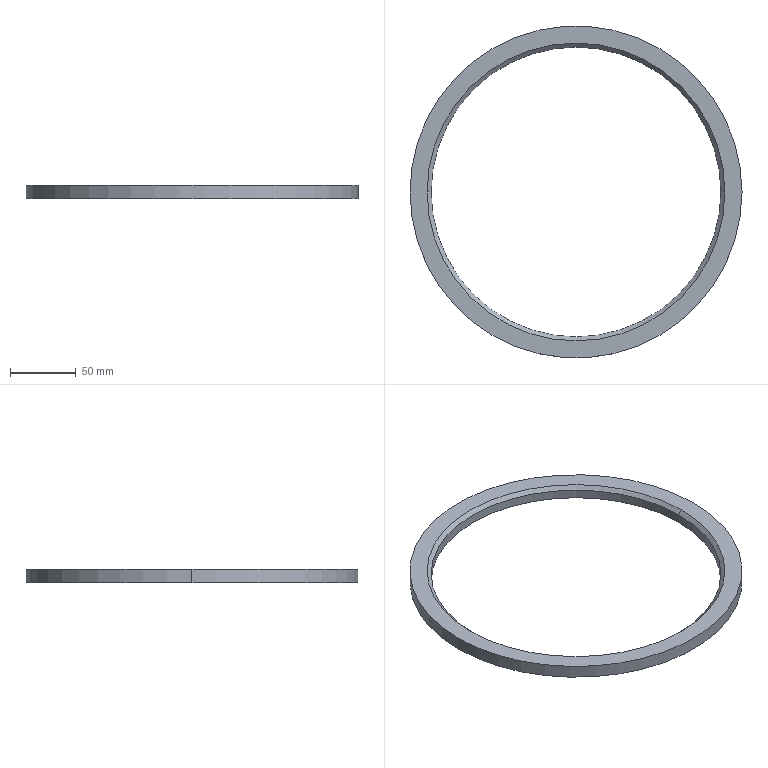Part | SolidWorks | features Chamfer 1, Extrusion 1 | 1 solid | 8 faces | box 252 x 252 x 10 mm | volume 115488 mm3 | cylinder 4 | cone 2 | plane 2 | commonest cylinder face diameters 220 x2 252 x2
STEP:
#1=CARTESIAN_POINT('',(-110.,0.,7.));
#2=VERTEX_POINT('',#1);
#3=CARTESIAN_POINT('',(110.,0.,7.));
#4=VERTEX_POINT('',#3);
#5=CARTESIAN_POINT('',(0.,0.,7.));
#6=DIRECTION('',(0.,0.,1.));
#7=DIRECTION('',(1.,0.,0.));
#8=AXIS2_PLACEMENT_3D('',#5,#6,#7);
#9=CIRCLE('',#8,110.);
#10=EDGE_CURVE('',#2,#4,#9,.T.);
#11=ORIENTED_EDGE('',*,*,#10,.F.);
#12=CARTESIAN_POINT('',(-113.,0.,10.));
#13=VERTEX_POINT('',#12);
#14=CARTESIAN_POINT('',(-110.,0.,7.));
#15=DIRECTION('',(-0.7071,0.,0.7071));
#16=VECTOR('',#15,1000.);
#17=LINE('',#14,#16);
#18=EDGE_CURVE('',#2,#13,#17,.T.);
#19=ORIENTED_EDGE('',*,*,#18,.T.);
#20=CARTESIAN_POINT('',(113.,0.,10.));
#21=VERTEX_POINT('',#20);
#22=CARTESIAN_POINT('',(0.,0.,10.));
#23=DIRECTION('',(0.,0.,-1.));
#24=DIRECTION('',(1.,0.,0.));
#25=AXIS2_PLACEMENT_3D('',#22,#23,#24);
#26=CIRCLE('',#25,113.);
#27=EDGE_CURVE('',#21,#13,#26,.T.);
#28=ORIENTED_EDGE('',*,*,#27,.F.);
#29=CARTESIAN_POINT('',(110.,0.,7.));
#30=DIRECTION('',(0.7071,0.,0.7071));
#31=VECTOR('',#30,1000.);
#32=LINE('',#29,#31);
#33=EDGE_CURVE('',#4,#21,#32,.T.);
#34=ORIENTED_EDGE('',*,*,#33,.F.);
#35=EDGE_LOOP('',(#11,#19,#28,#34));
#36=FACE_OUTER_BOUND('',#35,.T.);
#37=CARTESIAN_POINT('',(0.,0.,7.));
#38=DIRECTION('',(0.,0.,1.));
#39=DIRECTION('',(1.,0.,0.));
#40=AXIS2_PLACEMENT_3D('',#37,#38,#39);
#41=CONICAL_SURFACE('',#40,110.,0.7854);
#42=ADVANCED_FACE('',(#36),#41,.F.);
#43=ORIENTED_EDGE('',*,*,#10,.T.);
#44=CARTESIAN_POINT('',(110.,0.,0.));
#45=VERTEX_POINT('',#44);
#46=CARTESIAN_POINT('',(110.,0.,10.));
#47=DIRECTION('',(0.,0.,-1.));
#48=VECTOR('',#47,1000.);
#49=LINE('',#46,#48);
#50=EDGE_CURVE('',#4,#45,#49,.T.);
#51=ORIENTED_EDGE('',*,*,#50,.T.);
#52=CARTESIAN_POINT('',(-110.,0.,0.));
#53=VERTEX_POINT('',#52);
#54=CARTESIAN_POINT('',(0.,0.,0.));
#55=DIRECTION('',(0.,0.,1.));
#56=DIRECTION('',(1.,0.,0.));
#57=AXIS2_PLACEMENT_3D('',#54,#55,#56);
#58=CIRCLE('',#57,110.);
#59=EDGE_CURVE('',#53,#45,#58,.T.);
#60=ORIENTED_EDGE('',*,*,#59,.F.);
#61=CARTESIAN_POINT('',(-110.,0.,10.));
#62=DIRECTION('',(0.,0.,-1.));
#63=VECTOR('',#62,1000.);
#64=LINE('',#61,#63);
#65=EDGE_CURVE('',#2,#53,#64,.T.);
#66=ORIENTED_EDGE('',*,*,#65,.F.);
#67=EDGE_LOOP('',(#43,#51,#60,#66));
#68=FACE_OUTER_BOUND('',#67,.T.);
#69=CARTESIAN_POINT('',(0.,0.,10.));
#70=DIRECTION('',(0.,0.,-1.));
#71=DIRECTION('',(-1.,0.,0.));
#72=AXIS2_PLACEMENT_3D('',#69,#70,#71);
#73=CYLINDRICAL_SURFACE('',#72,110.);
#74=ADVANCED_FACE('',(#68),#73,.F.);
#75=CARTESIAN_POINT('',(126.,0.,10.));
#76=VERTEX_POINT('',#75);
#77=CARTESIAN_POINT('',(-126.,0.,10.));
#78=VERTEX_POINT('',#77);
#79=CARTESIAN_POINT('',(0.,0.,10.));
#80=DIRECTION('',(0.,0.,1.));
#81=DIRECTION('',(1.,0.,0.));
#82=AXIS2_PLACEMENT_3D('',#79,#80,#81);
#83=CIRCLE('',#82,126.);
#84=EDGE_CURVE('',#76,#78,#83,.T.);
#85=ORIENTED_EDGE('',*,*,#84,.F.);
#86=CARTESIAN_POINT('',(126.,0.,0.));
#87=VERTEX_POINT('',#86);
#88=CARTESIAN_POINT('',(126.,0.,10.));
#89=DIRECTION('',(0.,0.,-1.));
#90=VECTOR('',#89,1000.);
#91=LINE('',#88,#90);
#92=EDGE_CURVE('',#76,#87,#91,.T.);
#93=ORIENTED_EDGE('',*,*,#92,.T.);
#94=CARTESIAN_POINT('',(-126.,0.,0.));
#95=VERTEX_POINT('',#94);
#96=CARTESIAN_POINT('',(0.,0.,0.));
#97=DIRECTION('',(0.,0.,1.));
#98=DIRECTION('',(1.,0.,0.));
#99=AXIS2_PLACEMENT_3D('',#96,#97,#98);
#100=CIRCLE('',#99,126.);
#101=EDGE_CURVE('',#87,#95,#100,.T.);
#102=ORIENTED_EDGE('',*,*,#101,.T.);
#103=CARTESIAN_POINT('',(-126.,0.,10.));
#104=DIRECTION('',(0.,0.,-1.));
#105=VECTOR('',#104,1000.);
#106=LINE('',#103,#105);
#107=EDGE_CURVE('',#78,#95,#106,.T.);
#108=ORIENTED_EDGE('',*,*,#107,.F.);
#109=EDGE_LOOP('',(#85,#93,#102,#108));
#110=FACE_OUTER_BOUND('',#109,.T.);
#111=CARTESIAN_POINT('',(0.,0.,10.));
#112=DIRECTION('',(0.,0.,-1.));
#113=DIRECTION('',(-1.,0.,0.));
#114=AXIS2_PLACEMENT_3D('',#111,#112,#113);
#115=CYLINDRICAL_SURFACE('',#114,126.);
#116=ADVANCED_FACE('',(#110),#115,.T.);
#117=ORIENTED_EDGE('',*,*,#27,.T.);
#118=CARTESIAN_POINT('',(0.,0.,10.));
#119=DIRECTION('',(0.,0.,-1.));
#120=DIRECTION('',(1.,0.,0.));
#121=AXIS2_PLACEMENT_3D('',#118,#119,#120);
#122=CIRCLE('',#121,113.);
#123=EDGE_CURVE('',#13,#21,#122,.T.);
#124=ORIENTED_EDGE('',*,*,#123,.T.);
#125=EDGE_LOOP('',(#117,#124));
#126=FACE_BOUND('',#125,.T.);
#127=CARTESIAN_POINT('',(0.,0.,10.));
#128=DIRECTION('',(0.,0.,1.));
#129=DIRECTION('',(1.,0.,0.));
#130=AXIS2_PLACEMENT_3D('',#127,#128,#129);
#131=CIRCLE('',#130,126.);
#132=EDGE_CURVE('',#78,#76,#131,.T.);
#133=ORIENTED_EDGE('',*,*,#132,.T.);
#134=ORIENTED_EDGE('',*,*,#84,.T.);
#135=EDGE_LOOP('',(#133,#134));
#136=FACE_OUTER_BOUND('',#135,.T.);
#137=CARTESIAN_POINT('',(0.,0.,10.));
#138=DIRECTION('',(0.,0.,1.));
#139=DIRECTION('',(1.,0.,0.));
#140=AXIS2_PLACEMENT_3D('',#137,#138,#139);
#141=PLANE('',#140);
#142=ADVANCED_FACE('',(#126,#136),#141,.T.);
#143=CARTESIAN_POINT('',(0.,0.,0.));
#144=DIRECTION('',(0.,0.,1.));
#145=DIRECTION('',(1.,0.,0.));
#146=AXIS2_PLACEMENT_3D('',#143,#144,#145);
#147=CIRCLE('',#146,126.);
#148=EDGE_CURVE('',#95,#87,#147,.T.);
#149=ORIENTED_EDGE('',*,*,#148,.F.);
#150=ORIENTED_EDGE('',*,*,#101,.F.);
#151=EDGE_LOOP('',(#149,#150));
#152=FACE_OUTER_BOUND('',#151,.T.);
#153=ORIENTED_EDGE('',*,*,#59,.T.);
#154=CARTESIAN_POINT('',(0.,0.,0.));
#155=DIRECTION('',(0.,0.,1.));
#156=DIRECTION('',(1.,0.,0.));
#157=AXIS2_PLACEMENT_3D('',#154,#155,#156);
#158=CIRCLE('',#157,110.);
#159=EDGE_CURVE('',#45,#53,#158,.T.);
#160=ORIENTED_EDGE('',*,*,#159,.T.);
#161=EDGE_LOOP('',(#153,#160));
#162=FACE_BOUND('',#161,.T.);
#163=CARTESIAN_POINT('',(0.,0.,0.));
#164=DIRECTION('',(0.,0.,1.));
#165=DIRECTION('',(1.,0.,0.));
#166=AXIS2_PLACEMENT_3D('',#163,#164,#165);
#167=PLANE('',#166);
#168=ADVANCED_FACE('',(#152,#162),#167,.F.);
#169=ORIENTED_EDGE('',*,*,#92,.F.);
#170=ORIENTED_EDGE('',*,*,#132,.F.);
#171=ORIENTED_EDGE('',*,*,#107,.T.);
#172=ORIENTED_EDGE('',*,*,#148,.T.);
#173=EDGE_LOOP('',(#169,#170,#171,#172));
#174=FACE_OUTER_BOUND('',#173,.T.);
#175=CARTESIAN_POINT('',(0.,0.,10.));
#176=DIRECTION('',(0.,0.,-1.));
#177=DIRECTION('',(-1.,0.,0.));
#178=AXIS2_PLACEMENT_3D('',#175,#176,#177);
#179=CYLINDRICAL_SURFACE('',#178,126.);
#180=ADVANCED_FACE('',(#174),#179,.T.);
#181=ORIENTED_EDGE('',*,*,#50,.F.);
#182=CARTESIAN_POINT('',(0.,0.,7.));
#183=DIRECTION('',(0.,0.,1.));
#184=DIRECTION('',(1.,0.,0.));
#185=AXIS2_PLACEMENT_3D('',#182,#183,#184);
#186=CIRCLE('',#185,110.);
#187=EDGE_CURVE('',#4,#2,#186,.T.);
#188=ORIENTED_EDGE('',*,*,#187,.T.);
#189=ORIENTED_EDGE('',*,*,#65,.T.);
#190=ORIENTED_EDGE('',*,*,#159,.F.);
#191=EDGE_LOOP('',(#181,#188,#189,#190));
#192=FACE_OUTER_BOUND('',#191,.T.);
#193=CARTESIAN_POINT('',(0.,0.,10.));
#194=DIRECTION('',(0.,0.,-1.));
#195=DIRECTION('',(-1.,0.,0.));
#196=AXIS2_PLACEMENT_3D('',#193,#194,#195);
#197=CYLINDRICAL_SURFACE('',#196,110.);
#198=ADVANCED_FACE('',(#192),#197,.F.);
#199=ORIENTED_EDGE('',*,*,#18,.F.);
#200=ORIENTED_EDGE('',*,*,#187,.F.);
#201=ORIENTED_EDGE('',*,*,#33,.T.);
#202=ORIENTED_EDGE('',*,*,#123,.F.);
#203=EDGE_LOOP('',(#199,#200,#201,#202));
#204=FACE_OUTER_BOUND('',#203,.T.);
#205=CARTESIAN_POINT('',(0.,0.,7.));
#206=DIRECTION('',(0.,0.,1.));
#207=DIRECTION('',(1.,0.,0.));
#208=AXIS2_PLACEMENT_3D('',#205,#206,#207);
#209=CONICAL_SURFACE('',#208,110.,0.7854);
#210=ADVANCED_FACE('',(#204),#209,.F.);
#211=CLOSED_SHELL('',(#42,#74,#116,#142,#168,#180,#198,#210));
#212=MANIFOLD_SOLID_BREP('',#211);
#213=CARTESIAN_POINT('',(0.,0.,0.));
#214=DIRECTION('',(0.,0.,1.));
#215=DIRECTION('',(1.,0.,0.));
#216=AXIS2_PLACEMENT_3D('',#213,#214,#215);
#217=(LENGTH_UNIT()NAMED_UNIT(*)SI_UNIT(.MILLI.,.METRE.));
#218=UNCERTAINTY_MEASURE_WITH_UNIT(LENGTH_MEASURE(0.00001),#217,'','');
#219=(NAMED_UNIT(*)PLANE_ANGLE_UNIT()SI_UNIT($,.RADIAN.));
#220=(NAMED_UNIT(*)SI_UNIT($,.STERADIAN.)SOLID_ANGLE_UNIT());
#221=(GEOMETRIC_REPRESENTATION_CONTEXT(3)GLOBAL_UNCERTAINTY_ASSIGNED_CONTEXT((#218))GLOBAL_UNIT_ASSIGNED_CONTEXT((#217,#219,#220))REPRESENTATION_CONTEXT('',''));
#222=ADVANCED_BREP_SHAPE_REPRESENTATION('',(#212,#216),#221);